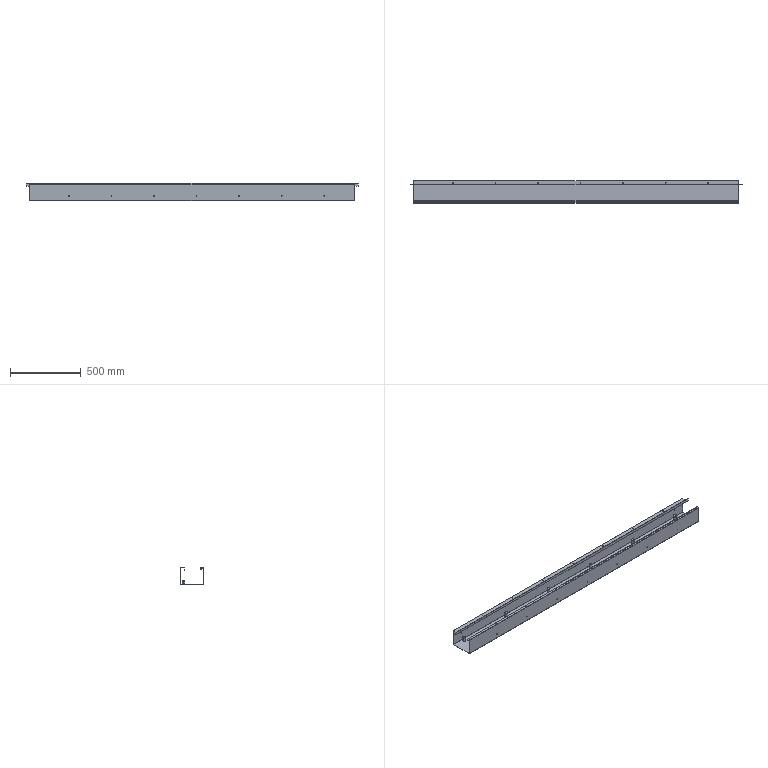Part | STEP file | SX-004-02 | 1 solid | 164 faces | box 2341 x 159.5 x 122 mm | volume 2176769 mm3 | cylinder 96 | plane 56 | cone 12 | commonest cylinder face diameters 5.4 x42 8.5 x12 12.5 x12 20 x12 0.4 x6 4.4 x6